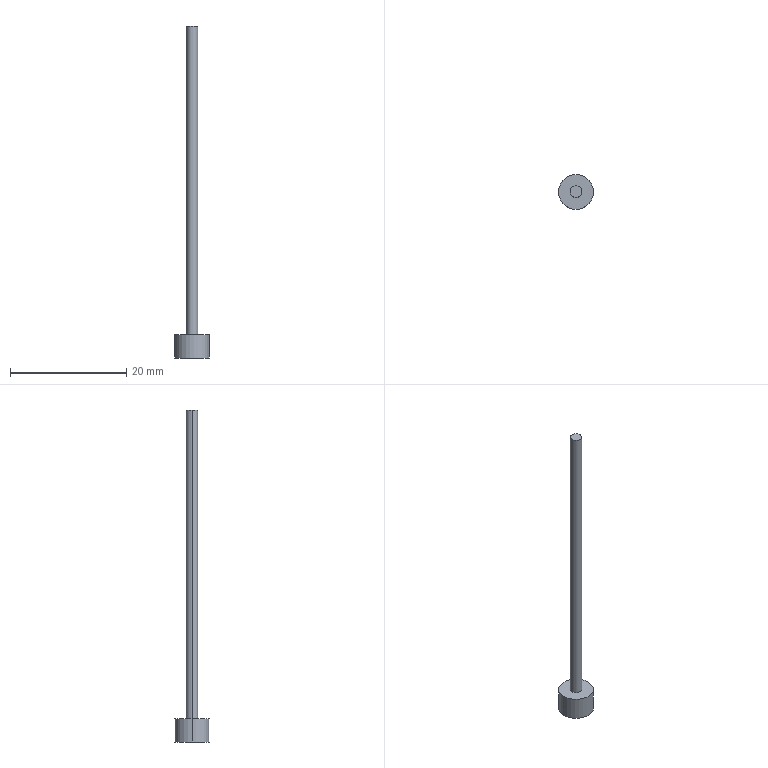Part | Creo | 1 solid | 48 faces | box 6 x 6 x 57.137 mm | volume 279.637 mm3 | other 27 | plane 16 | cylinder 5 | commonest cylinder face diameters 2 x2 6 x2 8.591 x1